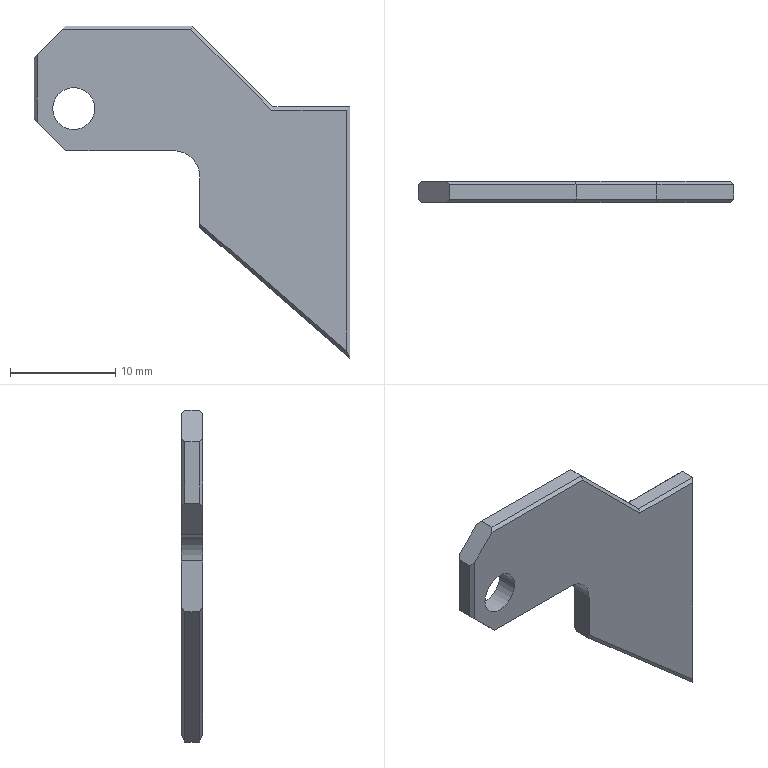Part | NX | 1 solid | 27 faces | box 30 x 2 x 31.579 mm | volume 877.917 mm3 | plane 24 | cylinder 3 | commonest cylinder face diameters 4 x2 5 x1
STEP:
#1=CARTESIAN_POINT('',(-137.75,158.2,-58.092));
#2=VERTEX_POINT('',#1);
#3=CARTESIAN_POINT('',(-123.5,158.2,-70.479));
#4=VERTEX_POINT('',#3);
#5=CARTESIAN_POINT('',(-130.625,158.2,-64.285));
#6=DIRECTION('',(0.7547,0.,-0.6561));
#7=VECTOR('',#6,1000.);
#8=LINE('',#5,#7);
#9=EDGE_CURVE('',#2,#4,#8,.T.);
#10=ORIENTED_EDGE('',*,*,#9,.T.);
#11=CARTESIAN_POINT('',(-123.5,156.8,-70.479));
#12=VERTEX_POINT('',#11);
#13=CARTESIAN_POINT('',(-123.5,156.5,-70.479));
#14=DIRECTION('',(0.,-1.,0.));
#15=VECTOR('',#14,1000.);
#16=LINE('',#13,#15);
#17=EDGE_CURVE('',#4,#12,#16,.T.);
#18=ORIENTED_EDGE('',*,*,#17,.T.);
#19=CARTESIAN_POINT('',(-137.75,156.8,-58.092));
#20=VERTEX_POINT('',#19);
#21=CARTESIAN_POINT('',(-130.625,156.8,-64.285));
#22=DIRECTION('',(0.7547,0.,-0.6561));
#23=VECTOR('',#22,1000.);
#24=LINE('',#21,#23);
#25=EDGE_CURVE('',#20,#12,#24,.T.);
#26=ORIENTED_EDGE('',*,*,#25,.F.);
#27=CARTESIAN_POINT('',(-137.75,156.5,-58.092));
#28=DIRECTION('',(0.,-1.,0.));
#29=VECTOR('',#28,1000.);
#30=LINE('',#27,#29);
#31=EDGE_CURVE('',#2,#20,#30,.T.);
#32=ORIENTED_EDGE('',*,*,#31,.F.);
#33=EDGE_LOOP('',(#10,#18,#26,#32));
#34=FACE_BOUND('',#33,.T.);
#35=CARTESIAN_POINT('',(-120.431,156.3,-73.147));
#36=DIRECTION('',(0.6561,0.,0.7547));
#37=DIRECTION('',(0.,-1.,0.));
#38=AXIS2_PLACEMENT_3D('',#35,#36,#37);
#39=PLANE('',#38);
#40=ADVANCED_FACE('',(#34),#39,.F.);
#41=CARTESIAN_POINT('',(-123.5,158.2,-46.6));
#42=VERTEX_POINT('',#41);
#43=CARTESIAN_POINT('',(-123.5,156.8,-46.6));
#44=VERTEX_POINT('',#43);
#45=CARTESIAN_POINT('',(-123.5,156.5,-46.6));
#46=DIRECTION('',(0.,-1.,0.));
#47=VECTOR('',#46,1000.);
#48=LINE('',#45,#47);
#49=EDGE_CURVE('',#42,#44,#48,.T.);
#50=ORIENTED_EDGE('',*,*,#49,.F.);
#51=CARTESIAN_POINT('',(-130.8,158.2,-46.6));
#52=VERTEX_POINT('',#51);
#53=CARTESIAN_POINT('',(-127.512,158.2,-46.6));
#54=DIRECTION('',(1.,0.,0.));
#55=VECTOR('',#54,1000.);
#56=LINE('',#53,#55);
#57=EDGE_CURVE('',#52,#42,#56,.T.);
#58=ORIENTED_EDGE('',*,*,#57,.F.);
#59=CARTESIAN_POINT('',(-130.8,156.8,-46.6));
#60=VERTEX_POINT('',#59);
#61=CARTESIAN_POINT('',(-130.8,156.5,-46.6));
#62=DIRECTION('',(0.,-1.,0.));
#63=VECTOR('',#62,1000.);
#64=LINE('',#61,#63);
#65=EDGE_CURVE('',#52,#60,#64,.T.);
#66=ORIENTED_EDGE('',*,*,#65,.T.);
#67=CARTESIAN_POINT('',(-127.512,156.8,-46.6));
#68=DIRECTION('',(1.,0.,0.));
#69=VECTOR('',#68,1000.);
#70=LINE('',#67,#69);
#71=EDGE_CURVE('',#60,#44,#70,.T.);
#72=ORIENTED_EDGE('',*,*,#71,.T.);
#73=EDGE_LOOP('',(#50,#58,#66,#72));
#74=FACE_BOUND('',#73,.T.);
#75=CARTESIAN_POINT('',(-133.5,158.5,-46.6));
#76=DIRECTION('',(0.,0.,1.));
#77=DIRECTION('',(0.,-1.,0.));
#78=AXIS2_PLACEMENT_3D('',#75,#76,#77);
#79=PLANE('',#78);
#80=ADVANCED_FACE('',(#74),#79,.T.);
#81=CARTESIAN_POINT('',(-153.5,156.8,-47.763));
#82=VERTEX_POINT('',#81);
#83=CARTESIAN_POINT('',(-153.5,156.8,-41.9));
#84=VERTEX_POINT('',#83);
#85=CARTESIAN_POINT('',(-153.5,156.8,-44.831));
#86=DIRECTION('',(0.,0.,1.));
#87=VECTOR('',#86,1000.);
#88=LINE('',#85,#87);
#89=EDGE_CURVE('',#82,#84,#88,.T.);
#90=ORIENTED_EDGE('',*,*,#89,.T.);
#91=CARTESIAN_POINT('',(-153.5,158.2,-41.9));
#92=VERTEX_POINT('',#91);
#93=CARTESIAN_POINT('',(-153.5,157.5,-41.9));
#94=DIRECTION('',(0.,-1.,0.));
#95=VECTOR('',#94,1000.);
#96=LINE('',#93,#95);
#97=EDGE_CURVE('',#92,#84,#96,.T.);
#98=ORIENTED_EDGE('',*,*,#97,.F.);
#99=CARTESIAN_POINT('',(-153.5,158.2,-47.763));
#100=VERTEX_POINT('',#99);
#101=CARTESIAN_POINT('',(-153.5,158.2,-44.831));
#102=DIRECTION('',(0.,0.,1.));
#103=VECTOR('',#102,1000.);
#104=LINE('',#101,#103);
#105=EDGE_CURVE('',#100,#92,#104,.T.);
#106=ORIENTED_EDGE('',*,*,#105,.F.);
#107=CARTESIAN_POINT('',(-153.5,157.5,-47.763));
#108=DIRECTION('',(0.,-1.,0.));
#109=VECTOR('',#108,1000.);
#110=LINE('',#107,#109);
#111=EDGE_CURVE('',#100,#82,#110,.T.);
#112=ORIENTED_EDGE('',*,*,#111,.T.);
#113=EDGE_LOOP('',(#90,#98,#106,#112));
#114=FACE_BOUND('',#113,.T.);
#115=CARTESIAN_POINT('',(-153.5,156.5,-42.9));
#116=DIRECTION('',(-1.,0.,0.));
#117=DIRECTION('',(0.,0.,1.));
#118=AXIS2_PLACEMENT_3D('',#115,#116,#117);
#119=PLANE('',#118);
#120=ADVANCED_FACE('',(#114),#119,.T.);
#121=CARTESIAN_POINT('',(-150.5,158.5,-50.763));
#122=VERTEX_POINT('',#121);
#123=CARTESIAN_POINT('',(-150.5,156.5,-50.763));
#124=VERTEX_POINT('',#123);
#125=CARTESIAN_POINT('',(-150.5,157.5,-50.763));
#126=DIRECTION('',(0.,-1.,0.));
#127=VECTOR('',#126,1000.);
#128=LINE('',#125,#127);
#129=EDGE_CURVE('',#122,#124,#128,.T.);
#130=ORIENTED_EDGE('',*,*,#129,.F.);
#131=CARTESIAN_POINT('',(-140.25,158.5,-50.763));
#132=VERTEX_POINT('',#131);
#133=CARTESIAN_POINT('',(-108.092,158.5,-50.763));
#134=DIRECTION('',(1.,0.,0.));
#135=VECTOR('',#134,1000.);
#136=LINE('',#133,#135);
#137=EDGE_CURVE('',#122,#132,#136,.T.);
#138=ORIENTED_EDGE('',*,*,#137,.T.);
#139=CARTESIAN_POINT('',(-140.25,156.5,-50.763));
#140=VERTEX_POINT('',#139);
#141=CARTESIAN_POINT('',(-140.25,156.5,-50.763));
#142=DIRECTION('',(0.,-1.,0.));
#143=VECTOR('',#142,1000.);
#144=LINE('',#141,#143);
#145=EDGE_CURVE('',#132,#140,#144,.T.);
#146=ORIENTED_EDGE('',*,*,#145,.T.);
#147=CARTESIAN_POINT('',(-108.092,156.5,-50.763));
#148=DIRECTION('',(1.,0.,0.));
#149=VECTOR('',#148,1000.);
#150=LINE('',#147,#149);
#151=EDGE_CURVE('',#124,#140,#150,.T.);
#152=ORIENTED_EDGE('',*,*,#151,.F.);
#153=EDGE_LOOP('',(#130,#138,#146,#152));
#154=FACE_BOUND('',#153,.T.);
#155=CARTESIAN_POINT('',(-137.75,156.3,-50.763));
#156=DIRECTION('',(0.,0.,1.));
#157=DIRECTION('',(0.,-1.,0.));
#158=AXIS2_PLACEMENT_3D('',#155,#156,#157);
#159=PLANE('',#158);
#160=ADVANCED_FACE('',(#154),#159,.F.);
#161=CARTESIAN_POINT('',(-151.75,158.5,-46.763));
#162=VERTEX_POINT('',#161);
#163=CARTESIAN_POINT('',(-147.75,158.5,-46.763));
#164=VERTEX_POINT('',#163);
#165=CARTESIAN_POINT('',(-149.75,158.5,-46.763));
#166=DIRECTION('',(0.,1.,0.));
#167=DIRECTION('',(-1.,0.,0.));
#168=AXIS2_PLACEMENT_3D('',#165,#166,#167);
#169=CIRCLE('',#168,2.);
#170=EDGE_CURVE('',#162,#164,#169,.T.);
#171=ORIENTED_EDGE('',*,*,#170,.T.);
#172=CARTESIAN_POINT('',(-147.75,156.5,-46.763));
#173=VERTEX_POINT('',#172);
#174=CARTESIAN_POINT('',(-147.75,156.3,-46.763));
#175=DIRECTION('',(0.,1.,0.));
#176=VECTOR('',#175,1000.);
#177=LINE('',#174,#176);
#178=EDGE_CURVE('',#173,#164,#177,.T.);
#179=ORIENTED_EDGE('',*,*,#178,.F.);
#180=CARTESIAN_POINT('',(-151.75,156.5,-46.763));
#181=VERTEX_POINT('',#180);
#182=CARTESIAN_POINT('',(-149.75,156.5,-46.763));
#183=DIRECTION('',(0.,1.,0.));
#184=DIRECTION('',(-1.,0.,0.));
#185=AXIS2_PLACEMENT_3D('',#182,#183,#184);
#186=CIRCLE('',#185,2.);
#187=EDGE_CURVE('',#181,#173,#186,.T.);
#188=ORIENTED_EDGE('',*,*,#187,.F.);
#189=CARTESIAN_POINT('',(-151.75,156.3,-46.763));
#190=DIRECTION('',(0.,1.,0.));
#191=VECTOR('',#190,1000.);
#192=LINE('',#189,#191);
#193=EDGE_CURVE('',#181,#162,#192,.T.);
#194=ORIENTED_EDGE('',*,*,#193,.T.);
#195=EDGE_LOOP('',(#171,#179,#188,#194));
#196=FACE_BOUND('',#195,.T.);
#197=CARTESIAN_POINT('',(-149.75,156.3,-46.763));
#198=DIRECTION('',(0.,1.,0.));
#199=DIRECTION('',(-1.,0.,0.));
#200=AXIS2_PLACEMENT_3D('',#197,#198,#199);
#201=CYLINDRICAL_SURFACE('',#200,2.);
#202=ADVANCED_FACE('',(#196),#201,.F.);
#203=CARTESIAN_POINT('',(-137.75,158.5,-53.263));
#204=VERTEX_POINT('',#203);
#205=CARTESIAN_POINT('',(-137.75,158.5,-57.694));
#206=VERTEX_POINT('',#205);
#207=CARTESIAN_POINT('',(-137.75,158.5,-58.685));
#208=DIRECTION('',(0.,0.,-1.));
#209=VECTOR('',#208,1000.);
#210=LINE('',#207,#209);
#211=EDGE_CURVE('',#204,#206,#210,.T.);
#212=ORIENTED_EDGE('',*,*,#211,.T.);
#213=CARTESIAN_POINT('',(-137.75,157.752,-58.685));
#214=DIRECTION('',(0.,-0.6024,-0.7982));
#215=VECTOR('',#214,1000.);
#216=LINE('',#213,#215);
#217=EDGE_CURVE('',#206,#2,#216,.T.);
#218=ORIENTED_EDGE('',*,*,#217,.T.);
#219=ORIENTED_EDGE('',*,*,#31,.T.);
#220=CARTESIAN_POINT('',(-137.75,156.5,-57.694));
#221=VERTEX_POINT('',#220);
#222=CARTESIAN_POINT('',(-137.75,157.248,-58.685));
#223=DIRECTION('',(0.,-0.6024,0.7982));
#224=VECTOR('',#223,1000.);
#225=LINE('',#222,#224);
#226=EDGE_CURVE('',#20,#221,#225,.T.);
#227=ORIENTED_EDGE('',*,*,#226,.T.);
#228=CARTESIAN_POINT('',(-137.75,156.5,-53.263));
#229=VERTEX_POINT('',#228);
#230=CARTESIAN_POINT('',(-137.75,156.5,-58.685));
#231=DIRECTION('',(0.,0.,-1.));
#232=VECTOR('',#231,1000.);
#233=LINE('',#230,#232);
#234=EDGE_CURVE('',#229,#221,#233,.T.);
#235=ORIENTED_EDGE('',*,*,#234,.F.);
#236=CARTESIAN_POINT('',(-137.75,156.5,-53.263));
#237=DIRECTION('',(0.,-1.,0.));
#238=VECTOR('',#237,1000.);
#239=LINE('',#236,#238);
#240=EDGE_CURVE('',#204,#229,#239,.T.);
#241=ORIENTED_EDGE('',*,*,#240,.F.);
#242=EDGE_LOOP('',(#212,#218,#219,#227,#235,#241));
#243=FACE_BOUND('',#242,.T.);
#244=CARTESIAN_POINT('',(-137.75,156.3,-58.463));
#245=DIRECTION('',(1.,0.,0.));
#246=DIRECTION('',(0.,1.,0.));
#247=AXIS2_PLACEMENT_3D('',#244,#245,#246);
#248=PLANE('',#247);
#249=ADVANCED_FACE('',(#243),#248,.F.);
#250=CARTESIAN_POINT('',(-130.924,158.5,-46.9));
#251=VERTEX_POINT('',#250);
#252=CARTESIAN_POINT('',(-123.8,158.5,-46.9));
#253=VERTEX_POINT('',#252);
#254=CARTESIAN_POINT('',(-127.512,158.5,-46.9));
#255=DIRECTION('',(1.,0.,0.));
#256=VECTOR('',#255,1000.);
#257=LINE('',#254,#256);
#258=EDGE_CURVE('',#251,#253,#257,.T.);
#259=ORIENTED_EDGE('',*,*,#258,.T.);
#260=CARTESIAN_POINT('',(-123.8,158.5,-69.821));
#261=VERTEX_POINT('',#260);
#262=CARTESIAN_POINT('',(-123.8,158.5,-58.685));
#263=DIRECTION('',(0.,0.,1.));
#264=VECTOR('',#263,1000.);
#265=LINE('',#262,#264);
#266=EDGE_CURVE('',#261,#253,#265,.T.);
#267=ORIENTED_EDGE('',*,*,#266,.F.);
#268=CARTESIAN_POINT('',(-130.428,158.5,-64.059));
#269=DIRECTION('',(0.7547,0.,-0.6561));
#270=VECTOR('',#269,1000.);
#271=LINE('',#268,#270);
#272=EDGE_CURVE('',#206,#261,#271,.T.);
#273=ORIENTED_EDGE('',*,*,#272,.F.);
#274=ORIENTED_EDGE('',*,*,#211,.F.);
#275=CARTESIAN_POINT('',(-140.25,158.5,-53.263));
#276=DIRECTION('',(0.,-1.,0.));
#277=DIRECTION('',(1.,0.,0.));
#278=AXIS2_PLACEMENT_3D('',#275,#276,#277);
#279=CIRCLE('',#278,2.5);
#280=EDGE_CURVE('',#204,#132,#279,.T.);
#281=ORIENTED_EDGE('',*,*,#280,.T.);
#282=ORIENTED_EDGE('',*,*,#137,.F.);
#283=CARTESIAN_POINT('',(-153.2,158.5,-48.063));
#284=VERTEX_POINT('',#283);
#285=CARTESIAN_POINT('',(-142.578,158.5,-58.685));
#286=DIRECTION('',(-0.7071,0.,0.7071));
#287=VECTOR('',#286,1000.);
#288=LINE('',#285,#287);
#289=EDGE_CURVE('',#122,#284,#288,.T.);
#290=ORIENTED_EDGE('',*,*,#289,.T.);
#291=CARTESIAN_POINT('',(-153.2,158.5,-41.6));
#292=VERTEX_POINT('',#291);
#293=CARTESIAN_POINT('',(-153.2,158.5,-44.831));
#294=DIRECTION('',(0.,0.,1.));
#295=VECTOR('',#294,1000.);
#296=LINE('',#293,#295);
#297=EDGE_CURVE('',#284,#292,#296,.T.);
#298=ORIENTED_EDGE('',*,*,#297,.T.);
#299=CARTESIAN_POINT('',(-150.8,158.5,-39.2));
#300=VERTEX_POINT('',#299);
#301=CARTESIAN_POINT('',(-170.285,158.5,-58.685));
#302=DIRECTION('',(-0.7071,0.,-0.7071));
#303=VECTOR('',#302,1000.);
#304=LINE('',#301,#303);
#305=EDGE_CURVE('',#300,#292,#304,.T.);
#306=ORIENTED_EDGE('',*,*,#305,.F.);
#307=CARTESIAN_POINT('',(-138.624,158.5,-39.2));
#308=VERTEX_POINT('',#307);
#309=CARTESIAN_POINT('',(-144.5,158.5,-39.2));
#310=DIRECTION('',(1.,0.,0.));
#311=VECTOR('',#310,1000.);
#312=LINE('',#309,#311);
#313=EDGE_CURVE('',#300,#308,#312,.T.);
#314=ORIENTED_EDGE('',*,*,#313,.T.);
#315=CARTESIAN_POINT('',(-119.139,158.5,-58.685));
#316=DIRECTION('',(-0.7071,0.,0.7071));
#317=VECTOR('',#316,1000.);
#318=LINE('',#315,#317);
#319=EDGE_CURVE('',#251,#308,#318,.T.);
#320=ORIENTED_EDGE('',*,*,#319,.F.);
#321=EDGE_LOOP('',(#259,#267,#273,#274,#281,#282,#290,#298,#306,#314,#320));
#322=FACE_BOUND('',#321,.T.);
#323=ORIENTED_EDGE('',*,*,#170,.F.);
#324=CARTESIAN_POINT('',(-149.75,158.5,-46.763));
#325=DIRECTION('',(0.,1.,0.));
#326=DIRECTION('',(-1.,0.,0.));
#327=AXIS2_PLACEMENT_3D('',#324,#325,#326);
#328=CIRCLE('',#327,2.);
#329=EDGE_CURVE('',#164,#162,#328,.T.);
#330=ORIENTED_EDGE('',*,*,#329,.F.);
#331=EDGE_LOOP('',(#323,#330));
#332=FACE_BOUND('',#331,.T.);
#333=CARTESIAN_POINT('',(-127.71,158.5,-52.75));
#334=DIRECTION('',(0.,1.,0.));
#335=DIRECTION('',(0.,0.,-1.));
#336=AXIS2_PLACEMENT_3D('',#333,#334,#335);
#337=PLANE('',#336);
#338=ADVANCED_FACE('',(#322,#332),#337,.T.);
#339=ORIENTED_EDGE('',*,*,#145,.F.);
#340=ORIENTED_EDGE('',*,*,#280,.F.);
#341=ORIENTED_EDGE('',*,*,#240,.T.);
#342=CARTESIAN_POINT('',(-140.25,156.5,-53.263));
#343=DIRECTION('',(0.,-1.,0.));
#344=DIRECTION('',(1.,0.,0.));
#345=AXIS2_PLACEMENT_3D('',#342,#343,#344);
#346=CIRCLE('',#345,2.5);
#347=EDGE_CURVE('',#229,#140,#346,.T.);
#348=ORIENTED_EDGE('',*,*,#347,.T.);
#349=EDGE_LOOP('',(#339,#340,#341,#348));
#350=FACE_BOUND('',#349,.T.);
#351=CARTESIAN_POINT('',(-140.25,156.5,-53.263));
#352=DIRECTION('',(0.,-1.,0.));
#353=DIRECTION('',(1.,0.,0.));
#354=AXIS2_PLACEMENT_3D('',#351,#352,#353);
#355=CYLINDRICAL_SURFACE('',#354,2.5);
#356=ADVANCED_FACE('',(#350),#355,.F.);
#357=ORIENTED_EDGE('',*,*,#129,.T.);
#358=CARTESIAN_POINT('',(-153.2,156.5,-48.063));
#359=VERTEX_POINT('',#358);
#360=CARTESIAN_POINT('',(-142.578,156.5,-58.685));
#361=DIRECTION('',(-0.7071,0.,0.7071));
#362=VECTOR('',#361,1000.);
#363=LINE('',#360,#362);
#364=EDGE_CURVE('',#124,#359,#363,.T.);
#365=ORIENTED_EDGE('',*,*,#364,.T.);
#366=CARTESIAN_POINT('',(-153.2,156.5,-48.063));
#367=DIRECTION('',(-0.5774,0.5774,0.5774));
#368=VECTOR('',#367,1000.);
#369=LINE('',#366,#368);
#370=EDGE_CURVE('',#359,#82,#369,.T.);
#371=ORIENTED_EDGE('',*,*,#370,.T.);
#372=ORIENTED_EDGE('',*,*,#111,.F.);
#373=CARTESIAN_POINT('',(-155.2,156.5,-46.063));
#374=DIRECTION('',(0.5774,0.5774,-0.5774));
#375=VECTOR('',#374,1000.);
#376=LINE('',#373,#375);
#377=EDGE_CURVE('',#100,#284,#376,.T.);
#378=ORIENTED_EDGE('',*,*,#377,.T.);
#379=ORIENTED_EDGE('',*,*,#289,.F.);
#380=EDGE_LOOP('',(#357,#365,#371,#372,#378,#379));
#381=FACE_BOUND('',#380,.T.);
#382=CARTESIAN_POINT('',(-152.,157.5,-49.263));
#383=DIRECTION('',(0.7071,0.,0.7071));
#384=DIRECTION('',(0.,-1.,0.));
#385=AXIS2_PLACEMENT_3D('',#382,#383,#384);
#386=PLANE('',#385);
#387=ADVANCED_FACE('',(#381),#386,.F.);
#388=CARTESIAN_POINT('',(-123.5,158.2,-58.685));
#389=DIRECTION('',(0.,0.,1.));
#390=VECTOR('',#389,1000.);
#391=LINE('',#388,#390);
#392=EDGE_CURVE('',#4,#42,#391,.T.);
#393=ORIENTED_EDGE('',*,*,#392,.T.);
#394=ORIENTED_EDGE('',*,*,#49,.T.);
#395=CARTESIAN_POINT('',(-123.5,156.8,-58.685));
#396=DIRECTION('',(0.,0.,-1.));
#397=VECTOR('',#396,1000.);
#398=LINE('',#395,#397);
#399=EDGE_CURVE('',#44,#12,#398,.T.);
#400=ORIENTED_EDGE('',*,*,#399,.T.);
#401=ORIENTED_EDGE('',*,*,#17,.F.);
#402=EDGE_LOOP('',(#393,#394,#400,#401));
#403=FACE_BOUND('',#402,.T.);
#404=CARTESIAN_POINT('',(-123.5,158.5,-45.6));
#405=DIRECTION('',(1.,0.,0.));
#406=DIRECTION('',(0.,1.,0.));
#407=AXIS2_PLACEMENT_3D('',#404,#405,#406);
#408=PLANE('',#407);
#409=ADVANCED_FACE('',(#403),#408,.T.);
#410=CARTESIAN_POINT('',(-135.585,170.285,-58.685));
#411=DIRECTION('',(-0.5774,0.5774,-0.5774));
#412=VECTOR('',#411,1000.);
#413=LINE('',#410,#412);
#414=EDGE_CURVE('',#42,#253,#413,.T.);
#415=ORIENTED_EDGE('',*,*,#414,.F.);
#416=ORIENTED_EDGE('',*,*,#392,.F.);
#417=CARTESIAN_POINT('',(-128.875,163.575,-58.685));
#418=DIRECTION('',(-0.3831,0.3831,0.8406));
#419=VECTOR('',#418,1000.);
#420=LINE('',#417,#419);
#421=EDGE_CURVE('',#4,#261,#420,.T.);
#422=ORIENTED_EDGE('',*,*,#421,.T.);
#423=ORIENTED_EDGE('',*,*,#266,.T.);
#424=EDGE_LOOP('',(#415,#416,#422,#423));
#425=FACE_BOUND('',#424,.T.);
#426=CARTESIAN_POINT('',(-123.65,158.35,-59.039));
#427=DIRECTION('',(0.7071,0.7071,0.));
#428=DIRECTION('',(0.,0.,-1.));
#429=AXIS2_PLACEMENT_3D('',#426,#427,#428);
#430=PLANE('',#429);
#431=ADVANCED_FACE('',(#425),#430,.T.);
#432=ORIENTED_EDGE('',*,*,#9,.F.);
#433=ORIENTED_EDGE('',*,*,#217,.F.);
#434=ORIENTED_EDGE('',*,*,#272,.T.);
#435=ORIENTED_EDGE('',*,*,#421,.F.);
#436=EDGE_LOOP('',(#432,#433,#434,#435));
#437=FACE_BOUND('',#436,.T.);
#438=CARTESIAN_POINT('',(-130.527,158.35,-64.172));
#439=DIRECTION('',(-0.4639,0.7071,-0.5337));
#440=DIRECTION('',(-0.7547,0.,0.6561));
#441=AXIS2_PLACEMENT_3D('',#438,#439,#440);
#442=PLANE('',#441);
#443=ADVANCED_FACE('',(#437),#442,.T.);
#444=ORIENTED_EDGE('',*,*,#89,.F.);
#445=ORIENTED_EDGE('',*,*,#370,.F.);
#446=CARTESIAN_POINT('',(-153.2,156.5,-41.6));
#447=VERTEX_POINT('',#446);
#448=CARTESIAN_POINT('',(-153.2,156.5,-44.831));
#449=DIRECTION('',(0.,0.,1.));
#450=VECTOR('',#449,1000.);
#451=LINE('',#448,#450);
#452=EDGE_CURVE('',#359,#447,#451,.T.);
#453=ORIENTED_EDGE('',*,*,#452,.T.);
#454=CARTESIAN_POINT('',(-153.2,156.5,-41.6));
#455=DIRECTION('',(-0.5774,0.5774,-0.5774));
#456=VECTOR('',#455,1000.);
#457=LINE('',#454,#456);
#458=EDGE_CURVE('',#447,#84,#457,.T.);
#459=ORIENTED_EDGE('',*,*,#458,.T.);
#460=EDGE_LOOP('',(#444,#445,#453,#459));
#461=FACE_BOUND('',#460,.T.);
#462=CARTESIAN_POINT('',(-153.35,156.65,-44.831));
#463=DIRECTION('',(-0.7071,-0.7071,0.));
#464=DIRECTION('',(-0.7071,0.7071,0.));
#465=AXIS2_PLACEMENT_3D('',#462,#463,#464);
#466=PLANE('',#465);
#467=ADVANCED_FACE('',(#461),#466,.T.);
#468=ORIENTED_EDGE('',*,*,#297,.F.);
#469=ORIENTED_EDGE('',*,*,#377,.F.);
#470=ORIENTED_EDGE('',*,*,#105,.T.);
#471=CARTESIAN_POINT('',(-155.2,156.5,-43.6));
#472=DIRECTION('',(0.5774,0.5774,0.5774));
#473=VECTOR('',#472,1000.);
#474=LINE('',#471,#473);
#475=EDGE_CURVE('',#92,#292,#474,.T.);
#476=ORIENTED_EDGE('',*,*,#475,.T.);
#477=EDGE_LOOP('',(#468,#469,#470,#476));
#478=FACE_BOUND('',#477,.T.);
#479=CARTESIAN_POINT('',(-153.35,158.35,-44.831));
#480=DIRECTION('',(-0.7071,0.7071,0.));
#481=DIRECTION('',(0.,0.,1.));
#482=AXIS2_PLACEMENT_3D('',#479,#480,#481);
#483=PLANE('',#482);
#484=ADVANCED_FACE('',(#478),#483,.T.);
#485=ORIENTED_EDGE('',*,*,#258,.F.);
#486=CARTESIAN_POINT('',(-135.806,170.285,-58.685));
#487=DIRECTION('',(-0.2811,0.6786,-0.6786));
#488=VECTOR('',#487,1000.);
#489=LINE('',#486,#488);
#490=EDGE_CURVE('',#52,#251,#489,.T.);
#491=ORIENTED_EDGE('',*,*,#490,.F.);
#492=ORIENTED_EDGE('',*,*,#57,.T.);
#493=ORIENTED_EDGE('',*,*,#414,.T.);
#494=EDGE_LOOP('',(#485,#491,#492,#493));
#495=FACE_BOUND('',#494,.T.);
#496=CARTESIAN_POINT('',(-127.512,158.35,-46.75));
#497=DIRECTION('',(0.,0.7071,0.7071));
#498=DIRECTION('',(1.,0.,0.));
#499=AXIS2_PLACEMENT_3D('',#496,#497,#498);
#500=PLANE('',#499);
#501=ADVANCED_FACE('',(#495),#500,.T.);
#502=CARTESIAN_POINT('',(-149.75,156.5,-46.763));
#503=DIRECTION('',(0.,1.,0.));
#504=DIRECTION('',(-1.,0.,0.));
#505=AXIS2_PLACEMENT_3D('',#502,#503,#504);
#506=CIRCLE('',#505,2.);
#507=EDGE_CURVE('',#173,#181,#506,.T.);
#508=ORIENTED_EDGE('',*,*,#507,.F.);
#509=ORIENTED_EDGE('',*,*,#178,.T.);
#510=ORIENTED_EDGE('',*,*,#329,.T.);
#511=ORIENTED_EDGE('',*,*,#193,.F.);
#512=EDGE_LOOP('',(#508,#509,#510,#511));
#513=FACE_BOUND('',#512,.T.);
#514=CARTESIAN_POINT('',(-149.75,156.3,-46.763));
#515=DIRECTION('',(0.,1.,0.));
#516=DIRECTION('',(-1.,0.,0.));
#517=AXIS2_PLACEMENT_3D('',#514,#515,#516);
#518=CYLINDRICAL_SURFACE('',#517,2.);
#519=ADVANCED_FACE('',(#513),#518,.F.);
#520=CARTESIAN_POINT('',(-130.924,156.5,-46.9));
#521=VERTEX_POINT('',#520);
#522=CARTESIAN_POINT('',(-123.8,156.5,-46.9));
#523=VERTEX_POINT('',#522);
#524=CARTESIAN_POINT('',(-127.512,156.5,-46.9));
#525=DIRECTION('',(1.,0.,0.));
#526=VECTOR('',#525,1000.);
#527=LINE('',#524,#526);
#528=EDGE_CURVE('',#521,#523,#527,.T.);
#529=ORIENTED_EDGE('',*,*,#528,.F.);
#530=CARTESIAN_POINT('',(-138.624,156.5,-39.2));
#531=VERTEX_POINT('',#530);
#532=CARTESIAN_POINT('',(-119.139,156.5,-58.685));
#533=DIRECTION('',(-0.7071,0.,0.7071));
#534=VECTOR('',#533,1000.);
#535=LINE('',#532,#534);
#536=EDGE_CURVE('',#521,#531,#535,.T.);
#537=ORIENTED_EDGE('',*,*,#536,.T.);
#538=CARTESIAN_POINT('',(-150.8,156.5,-39.2));
#539=VERTEX_POINT('',#538);
#540=CARTESIAN_POINT('',(-144.5,156.5,-39.2));
#541=DIRECTION('',(1.,0.,0.));
#542=VECTOR('',#541,1000.);
#543=LINE('',#540,#542);
#544=EDGE_CURVE('',#539,#531,#543,.T.);
#545=ORIENTED_EDGE('',*,*,#544,.F.);
#546=CARTESIAN_POINT('',(-170.285,156.5,-58.685));
#547=DIRECTION('',(-0.7071,0.,-0.7071));
#548=VECTOR('',#547,1000.);
#549=LINE('',#546,#548);
#550=EDGE_CURVE('',#539,#447,#549,.T.);
#551=ORIENTED_EDGE('',*,*,#550,.T.);
#552=ORIENTED_EDGE('',*,*,#452,.F.);
#553=ORIENTED_EDGE('',*,*,#364,.F.);
#554=ORIENTED_EDGE('',*,*,#151,.T.);
#555=ORIENTED_EDGE('',*,*,#347,.F.);
#556=ORIENTED_EDGE('',*,*,#234,.T.);
#557=CARTESIAN_POINT('',(-123.8,156.5,-69.821));
#558=VERTEX_POINT('',#557);
#559=CARTESIAN_POINT('',(-130.428,156.5,-64.059));
#560=DIRECTION('',(0.7547,0.,-0.6561));
#561=VECTOR('',#560,1000.);
#562=LINE('',#559,#561);
#563=EDGE_CURVE('',#221,#558,#562,.T.);
#564=ORIENTED_EDGE('',*,*,#563,.T.);
#565=CARTESIAN_POINT('',(-123.8,156.5,-58.685));
#566=DIRECTION('',(0.,0.,-1.));
#567=VECTOR('',#566,1000.);
#568=LINE('',#565,#567);
#569=EDGE_CURVE('',#523,#558,#568,.T.);
#570=ORIENTED_EDGE('',*,*,#569,.F.);
#571=EDGE_LOOP('',(#529,#537,#545,#551,#552,#553,#554,#555,#556,#564,#570));
#572=FACE_BOUND('',#571,.T.);
#573=ORIENTED_EDGE('',*,*,#507,.T.);
#574=ORIENTED_EDGE('',*,*,#187,.T.);
#575=EDGE_LOOP('',(#573,#574));
#576=FACE_BOUND('',#575,.T.);
#577=CARTESIAN_POINT('',(-127.71,156.5,-52.75));
#578=DIRECTION('',(0.,1.,0.));
#579=DIRECTION('',(0.,0.,-1.));
#580=AXIS2_PLACEMENT_3D('',#577,#578,#579);
#581=PLANE('',#580);
#582=ADVANCED_FACE('',(#572,#576),#581,.F.);
#583=CARTESIAN_POINT('',(-150.5,156.8,-38.9));
#584=VERTEX_POINT('',#583);
#585=CARTESIAN_POINT('',(-138.5,156.8,-38.9));
#586=VERTEX_POINT('',#585);
#587=CARTESIAN_POINT('',(-144.5,156.8,-38.9));
#588=DIRECTION('',(1.,0.,0.));
#589=VECTOR('',#588,1000.);
#590=LINE('',#587,#589);
#591=EDGE_CURVE('',#584,#586,#590,.T.);
#592=ORIENTED_EDGE('',*,*,#591,.T.);
#593=CARTESIAN_POINT('',(-138.5,158.2,-38.9));
#594=VERTEX_POINT('',#593);
#595=CARTESIAN_POINT('',(-138.5,157.5,-38.9));
#596=DIRECTION('',(0.,1.,0.));
#597=VECTOR('',#596,1000.);
#598=LINE('',#595,#597);
#599=EDGE_CURVE('',#586,#594,#598,.T.);
#600=ORIENTED_EDGE('',*,*,#599,.T.);
#601=CARTESIAN_POINT('',(-150.5,158.2,-38.9));
#602=VERTEX_POINT('',#601);
#603=CARTESIAN_POINT('',(-144.5,158.2,-38.9));
#604=DIRECTION('',(1.,0.,0.));
#605=VECTOR('',#604,1000.);
#606=LINE('',#603,#605);
#607=EDGE_CURVE('',#602,#594,#606,.T.);
#608=ORIENTED_EDGE('',*,*,#607,.F.);
#609=CARTESIAN_POINT('',(-150.5,157.5,-38.9));
#610=DIRECTION('',(0.,-1.,0.));
#611=VECTOR('',#610,1000.);
#612=LINE('',#609,#611);
#613=EDGE_CURVE('',#602,#584,#612,.T.);
#614=ORIENTED_EDGE('',*,*,#613,.T.);
#615=EDGE_LOOP('',(#592,#600,#608,#614));
#616=FACE_BOUND('',#615,.T.);
#617=CARTESIAN_POINT('',(-131.36,157.464,-38.9));
#618=DIRECTION('',(0.,0.,1.));
#619=DIRECTION('',(1.,0.,0.));
#620=AXIS2_PLACEMENT_3D('',#617,#618,#619);
#621=PLANE('',#620);
#622=ADVANCED_FACE('',(#616),#621,.T.);
#623=ORIENTED_EDGE('',*,*,#613,.F.);
#624=CARTESIAN_POINT('',(-148.8,156.5,-37.2));
#625=DIRECTION('',(-0.5774,0.5774,-0.5774));
#626=VECTOR('',#625,1000.);
#627=LINE('',#624,#626);
#628=EDGE_CURVE('',#602,#300,#627,.T.);
#629=ORIENTED_EDGE('',*,*,#628,.T.);
#630=ORIENTED_EDGE('',*,*,#305,.T.);
#631=ORIENTED_EDGE('',*,*,#475,.F.);
#632=ORIENTED_EDGE('',*,*,#97,.T.);
#633=ORIENTED_EDGE('',*,*,#458,.F.);
#634=ORIENTED_EDGE('',*,*,#550,.F.);
#635=CARTESIAN_POINT('',(-170.285,137.015,-58.685));
#636=DIRECTION('',(-0.5774,-0.5774,-0.5774));
#637=VECTOR('',#636,1000.);
#638=LINE('',#635,#637);
#639=EDGE_CURVE('',#584,#539,#638,.T.);
#640=ORIENTED_EDGE('',*,*,#639,.F.);
#641=EDGE_LOOP('',(#623,#629,#630,#631,#632,#633,#634,#640));
#642=FACE_BOUND('',#641,.T.);
#643=CARTESIAN_POINT('',(-152.,157.5,-40.4));
#644=DIRECTION('',(-0.7071,0.,0.7071));
#645=DIRECTION('',(0.,1.,0.));
#646=AXIS2_PLACEMENT_3D('',#643,#644,#645);
#647=PLANE('',#646);
#648=ADVANCED_FACE('',(#642),#647,.T.);
#649=CARTESIAN_POINT('',(-118.715,158.2,-58.685));
#650=DIRECTION('',(-0.7071,0.,0.7071));
#651=VECTOR('',#650,1000.);
#652=LINE('',#649,#651);
#653=EDGE_CURVE('',#52,#594,#652,.T.);
#654=ORIENTED_EDGE('',*,*,#653,.T.);
#655=ORIENTED_EDGE('',*,*,#599,.F.);
#656=CARTESIAN_POINT('',(-118.715,156.8,-58.685));
#657=DIRECTION('',(-0.7071,0.,0.7071));
#658=VECTOR('',#657,1000.);
#659=LINE('',#656,#658);
#660=EDGE_CURVE('',#60,#586,#659,.T.);
#661=ORIENTED_EDGE('',*,*,#660,.F.);
#662=ORIENTED_EDGE('',*,*,#65,.F.);
#663=EDGE_LOOP('',(#654,#655,#661,#662));
#664=FACE_BOUND('',#663,.T.);
#665=CARTESIAN_POINT('',(-131.,157.5,-46.4));
#666=DIRECTION('',(0.7071,0.,0.7071));
#667=DIRECTION('',(0.,-1.,0.));
#668=AXIS2_PLACEMENT_3D('',#665,#666,#667);
#669=PLANE('',#668);
#670=ADVANCED_FACE('',(#664),#669,.T.);
#671=ORIENTED_EDGE('',*,*,#399,.F.);
#672=CARTESIAN_POINT('',(-135.585,144.715,-58.685));
#673=DIRECTION('',(0.5774,0.5774,0.5774));
#674=VECTOR('',#673,1000.);
#675=LINE('',#672,#674);
#676=EDGE_CURVE('',#523,#44,#675,.T.);
#677=ORIENTED_EDGE('',*,*,#676,.F.);
#678=ORIENTED_EDGE('',*,*,#569,.T.);
#679=CARTESIAN_POINT('',(-128.875,151.425,-58.685));
#680=DIRECTION('',(-0.3831,-0.3831,0.8406));
#681=VECTOR('',#680,1000.);
#682=LINE('',#679,#681);
#683=EDGE_CURVE('',#12,#558,#682,.T.);
#684=ORIENTED_EDGE('',*,*,#683,.F.);
#685=EDGE_LOOP('',(#671,#677,#678,#684));
#686=FACE_BOUND('',#685,.T.);
#687=CARTESIAN_POINT('',(-123.65,156.65,-59.039));
#688=DIRECTION('',(-0.7071,0.7071,0.));
#689=DIRECTION('',(0.,0.,1.));
#690=AXIS2_PLACEMENT_3D('',#687,#688,#689);
#691=PLANE('',#690);
#692=ADVANCED_FACE('',(#686),#691,.F.);
#693=ORIENTED_EDGE('',*,*,#653,.F.);
#694=ORIENTED_EDGE('',*,*,#490,.T.);
#695=ORIENTED_EDGE('',*,*,#319,.T.);
#696=CARTESIAN_POINT('',(-137.796,156.5,-37.2));
#697=DIRECTION('',(0.2811,-0.6786,0.6786));
#698=VECTOR('',#697,1000.);
#699=LINE('',#696,#698);
#700=EDGE_CURVE('',#308,#594,#699,.T.);
#701=ORIENTED_EDGE('',*,*,#700,.T.);
#702=EDGE_LOOP('',(#693,#694,#695,#701));
#703=FACE_BOUND('',#702,.T.);
#704=CARTESIAN_POINT('',(-134.256,158.35,-43.356));
#705=DIRECTION('',(0.5,0.7071,0.5));
#706=DIRECTION('',(0.7071,0.,-0.7071));
#707=AXIS2_PLACEMENT_3D('',#704,#705,#706);
#708=PLANE('',#707);
#709=ADVANCED_FACE('',(#703),#708,.T.);
#710=ORIENTED_EDGE('',*,*,#607,.T.);
#711=ORIENTED_EDGE('',*,*,#700,.F.);
#712=ORIENTED_EDGE('',*,*,#313,.F.);
#713=ORIENTED_EDGE('',*,*,#628,.F.);
#714=EDGE_LOOP('',(#710,#711,#712,#713));
#715=FACE_BOUND('',#714,.T.);
#716=CARTESIAN_POINT('',(-144.5,158.35,-39.05));
#717=DIRECTION('',(0.,-0.7071,-0.7071));
#718=DIRECTION('',(0.,-0.7071,0.7071));
#719=AXIS2_PLACEMENT_3D('',#716,#717,#718);
#720=PLANE('',#719);
#721=ADVANCED_FACE('',(#715),#720,.F.);
#722=ORIENTED_EDGE('',*,*,#591,.F.);
#723=ORIENTED_EDGE('',*,*,#639,.T.);
#724=ORIENTED_EDGE('',*,*,#544,.T.);
#725=CARTESIAN_POINT('',(-146.695,137.015,-58.685));
#726=DIRECTION('',(-0.2811,-0.6786,-0.6786));
#727=VECTOR('',#726,1000.);
#728=LINE('',#725,#727);
#729=EDGE_CURVE('',#586,#531,#728,.T.);
#730=ORIENTED_EDGE('',*,*,#729,.F.);
#731=EDGE_LOOP('',(#722,#723,#724,#730));
#732=FACE_BOUND('',#731,.T.);
#733=CARTESIAN_POINT('',(-144.5,156.65,-39.05));
#734=DIRECTION('',(0.,-0.7071,0.7071));
#735=DIRECTION('',(-1.,0.,0.));
#736=AXIS2_PLACEMENT_3D('',#733,#734,#735);
#737=PLANE('',#736);
#738=ADVANCED_FACE('',(#732),#737,.T.);
#739=ORIENTED_EDGE('',*,*,#563,.F.);
#740=ORIENTED_EDGE('',*,*,#226,.F.);
#741=ORIENTED_EDGE('',*,*,#25,.T.);
#742=ORIENTED_EDGE('',*,*,#683,.T.);
#743=EDGE_LOOP('',(#739,#740,#741,#742));
#744=FACE_BOUND('',#743,.T.);
#745=CARTESIAN_POINT('',(-130.527,156.65,-64.172));
#746=DIRECTION('',(-0.4639,-0.7071,-0.5337));
#747=DIRECTION('',(0.,0.6024,-0.7982));
#748=AXIS2_PLACEMENT_3D('',#745,#746,#747);
#749=PLANE('',#748);
#750=ADVANCED_FACE('',(#744),#749,.T.);
#751=CARTESIAN_POINT('',(-135.806,144.715,-58.685));
#752=DIRECTION('',(0.2811,0.6786,0.6786));
#753=VECTOR('',#752,1000.);
#754=LINE('',#751,#753);
#755=EDGE_CURVE('',#521,#60,#754,.T.);
#756=ORIENTED_EDGE('',*,*,#755,.T.);
#757=ORIENTED_EDGE('',*,*,#660,.T.);
#758=ORIENTED_EDGE('',*,*,#729,.T.);
#759=ORIENTED_EDGE('',*,*,#536,.F.);
#760=EDGE_LOOP('',(#756,#757,#758,#759));
#761=FACE_BOUND('',#760,.T.);
#762=CARTESIAN_POINT('',(-134.256,156.65,-43.356));
#763=DIRECTION('',(-0.5,0.7071,-0.5));
#764=DIRECTION('',(-0.7071,0.,0.7071));
#765=AXIS2_PLACEMENT_3D('',#762,#763,#764);
#766=PLANE('',#765);
#767=ADVANCED_FACE('',(#761),#766,.F.);
#768=ORIENTED_EDGE('',*,*,#528,.T.);
#769=ORIENTED_EDGE('',*,*,#676,.T.);
#770=ORIENTED_EDGE('',*,*,#71,.F.);
#771=ORIENTED_EDGE('',*,*,#755,.F.);
#772=EDGE_LOOP('',(#768,#769,#770,#771));
#773=FACE_BOUND('',#772,.T.);
#774=CARTESIAN_POINT('',(-127.512,156.65,-46.75));
#775=DIRECTION('',(0.,0.7071,-0.7071));
#776=DIRECTION('',(-1.,0.,0.));
#777=AXIS2_PLACEMENT_3D('',#774,#775,#776);
#778=PLANE('',#777);
#779=ADVANCED_FACE('',(#773),#778,.F.);
#780=CLOSED_SHELL('',(#40,#80,#120,#160,#202,#249,#338,#356,#387,#409,#431,#443,#467,#484,#501,#519,#582,#622,#648,#670,#692,#709,#721,#738,#750,#767,#779));
#781=MANIFOLD_SOLID_BREP('',#780);
#782=(LENGTH_UNIT()NAMED_UNIT(*)SI_UNIT(.MILLI.,.METRE.));
#783=UNCERTAINTY_MEASURE_WITH_UNIT(LENGTH_MEASURE(0.00001),#782,'','');
#784=(NAMED_UNIT(*)PLANE_ANGLE_UNIT()SI_UNIT($,.RADIAN.));
#785=(NAMED_UNIT(*)SI_UNIT($,.STERADIAN.)SOLID_ANGLE_UNIT());
#786=(GEOMETRIC_REPRESENTATION_CONTEXT(3)GLOBAL_UNCERTAINTY_ASSIGNED_CONTEXT((#783))GLOBAL_UNIT_ASSIGNED_CONTEXT((#782,#784,#785))REPRESENTATION_CONTEXT('',''));
#787=ADVANCED_BREP_SHAPE_REPRESENTATION('',(#781),#786);